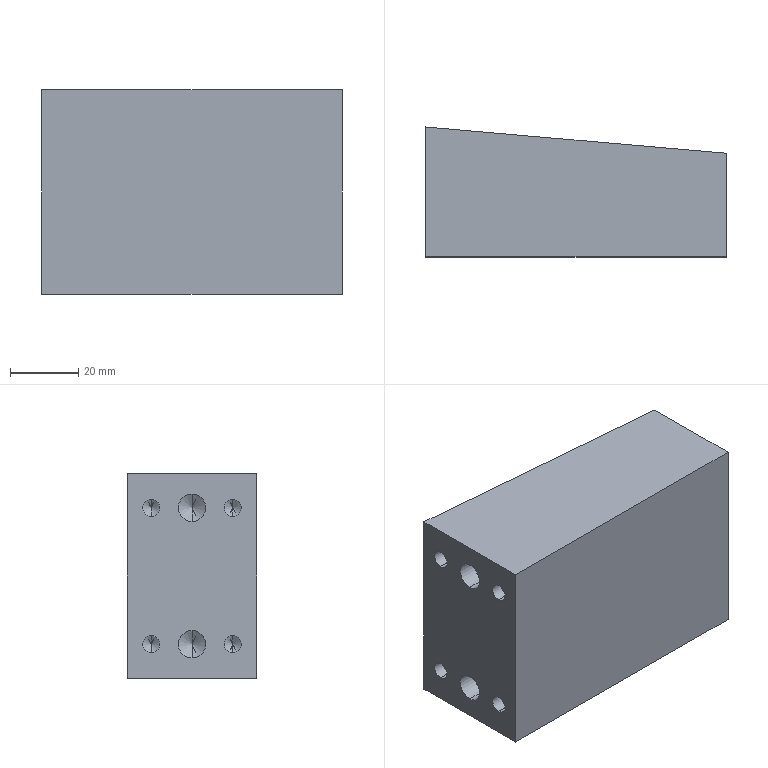Part | STEP file | OP10-134_cylinder stand (3) | 1 solid | 46 faces | box 88 x 38 x 60 mm | volume 176864 mm3 | cone 20 | cylinder 20 | plane 6 | commonest cylinder face diameters 4.2 x8 5 x8 8 x4